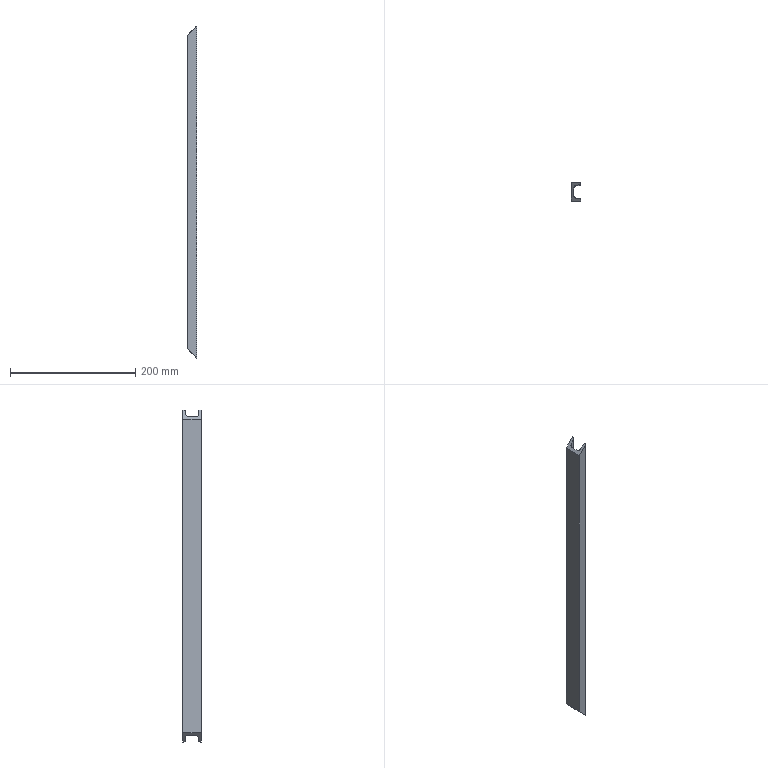Part | STEP file | DIN 1026-1 U 30x15 1785506883170 | 1 solid | 14 faces | box 15 x 30 x 530 mm | volume 112916 mm3 | plane 10 | cylinder 4 | commonest cylinder face diameters 4 x2 9 x2
STEP:
#1=CARTESIAN_POINT('',(13.159,10.953,-13.159));
#2=VERTEX_POINT('',#1);
#3=CARTESIAN_POINT('',(15.,12.946,-15.));
#4=VERTEX_POINT('',#3);
#5=CARTESIAN_POINT('',(13.,12.946,-13.));
#6=DIRECTION('',(0.7071,0.,0.7071));
#7=DIRECTION('',(-0.7071,0.,0.7071));
#8=AXIS2_PLACEMENT_3D('',#5,#6,#7);
#9=ELLIPSE('',#8,2.828,2.);
#10=EDGE_CURVE('',#2,#4,#9,.T.);
#11=ORIENTED_EDGE('',*,*,#10,.F.);
#12=CARTESIAN_POINT('',(8.141,10.551,-8.141));
#13=VERTEX_POINT('',#12);
#14=CARTESIAN_POINT('',(3.103,10.148,-3.103));
#15=DIRECTION('',(0.706,0.05648,-0.706));
#16=VECTOR('',#15,10.);
#17=LINE('',#14,#16);
#18=EDGE_CURVE('',#13,#2,#17,.T.);
#19=ORIENTED_EDGE('',*,*,#18,.F.);
#20=CARTESIAN_POINT('',(4.,6.066,-4.));
#21=VERTEX_POINT('',#20);
#22=CARTESIAN_POINT('',(8.5,6.066,-8.5));
#23=DIRECTION('',(-0.7071,0.,-0.7071));
#24=DIRECTION('',(-0.7071,0.,0.7071));
#25=AXIS2_PLACEMENT_3D('',#22,#23,#24);
#26=ELLIPSE('',#25,6.364,4.5);
#27=EDGE_CURVE('',#21,#13,#26,.T.);
#28=ORIENTED_EDGE('',*,*,#27,.F.);
#29=CARTESIAN_POINT('',(4.,-6.066,-4.));
#30=VERTEX_POINT('',#29);
#31=CARTESIAN_POINT('',(4.,0.,-4.));
#32=DIRECTION('',(0.,1.,0.));
#33=VECTOR('',#32,10.);
#34=LINE('',#31,#33);
#35=EDGE_CURVE('',#30,#21,#34,.T.);
#36=ORIENTED_EDGE('',*,*,#35,.F.);
#37=CARTESIAN_POINT('',(8.141,-10.551,-8.141));
#38=VERTEX_POINT('',#37);
#39=CARTESIAN_POINT('',(8.5,-6.066,-8.5));
#40=DIRECTION('',(-0.7071,0.,-0.7071));
#41=DIRECTION('',(-0.7071,0.,0.7071));
#42=AXIS2_PLACEMENT_3D('',#39,#40,#41);
#43=ELLIPSE('',#42,6.364,4.5);
#44=EDGE_CURVE('',#38,#30,#43,.T.);
#45=ORIENTED_EDGE('',*,*,#44,.F.);
#46=CARTESIAN_POINT('',(13.159,-10.953,-13.159));
#47=VERTEX_POINT('',#46);
#48=CARTESIAN_POINT('',(1.844,-10.048,-1.844));
#49=DIRECTION('',(-0.706,0.05648,0.706));
#50=VECTOR('',#49,10.);
#51=LINE('',#48,#50);
#52=EDGE_CURVE('',#47,#38,#51,.T.);
#53=ORIENTED_EDGE('',*,*,#52,.F.);
#54=CARTESIAN_POINT('',(15.,-12.946,-15.));
#55=VERTEX_POINT('',#54);
#56=CARTESIAN_POINT('',(13.,-12.946,-13.));
#57=DIRECTION('',(0.7071,0.,0.7071));
#58=DIRECTION('',(-0.7071,0.,0.7071));
#59=AXIS2_PLACEMENT_3D('',#56,#57,#58);
#60=ELLIPSE('',#59,2.828,2.);
#61=EDGE_CURVE('',#55,#47,#60,.T.);
#62=ORIENTED_EDGE('',*,*,#61,.F.);
#63=CARTESIAN_POINT('',(15.,-15.,-15.));
#64=VERTEX_POINT('',#63);
#65=CARTESIAN_POINT('',(15.,-6.473,-15.));
#66=DIRECTION('',(0.,-1.,0.));
#67=VECTOR('',#66,10.);
#68=LINE('',#65,#67);
#69=EDGE_CURVE('',#55,#64,#68,.T.);
#70=ORIENTED_EDGE('',*,*,#69,.T.);
#71=CARTESIAN_POINT('',(0.,-15.,0.));
#72=VERTEX_POINT('',#71);
#73=CARTESIAN_POINT('',(3.75,-15.,-3.75));
#74=DIRECTION('',(0.7071,0.,-0.7071));
#75=VECTOR('',#74,10.);
#76=LINE('',#73,#75);
#77=EDGE_CURVE('',#72,#64,#76,.T.);
#78=ORIENTED_EDGE('',*,*,#77,.F.);
#79=CARTESIAN_POINT('',(0.,15.,0.));
#80=VERTEX_POINT('',#79);
#81=CARTESIAN_POINT('',(0.,0.,0.));
#82=DIRECTION('',(0.,-1.,0.));
#83=VECTOR('',#82,10.);
#84=LINE('',#81,#83);
#85=EDGE_CURVE('',#80,#72,#84,.T.);
#86=ORIENTED_EDGE('',*,*,#85,.F.);
#87=CARTESIAN_POINT('',(15.,15.,-15.));
#88=VERTEX_POINT('',#87);
#89=CARTESIAN_POINT('',(0.,15.,0.));
#90=DIRECTION('',(-0.7071,0.,0.7071));
#91=VECTOR('',#90,10.);
#92=LINE('',#89,#91);
#93=EDGE_CURVE('',#88,#80,#92,.T.);
#94=ORIENTED_EDGE('',*,*,#93,.F.);
#95=CARTESIAN_POINT('',(15.,7.5,-15.));
#96=DIRECTION('',(0.,-1.,0.));
#97=VECTOR('',#96,10.);
#98=LINE('',#95,#97);
#99=EDGE_CURVE('',#88,#4,#98,.T.);
#100=ORIENTED_EDGE('',*,*,#99,.T.);
#101=EDGE_LOOP('',(#11,#19,#28,#36,#45,#53,#62,#70,#78,#86,#94,#100));
#102=FACE_OUTER_BOUND('',#101,.T.);
#103=CARTESIAN_POINT('',(0.,0.,0.));
#104=DIRECTION('',(0.7071,0.,0.7071));
#105=DIRECTION('',(0.7071,0.,-0.7071));
#106=AXIS2_PLACEMENT_3D('',#103,#104,#105);
#107=PLANE('',#106);
#108=ADVANCED_FACE('',(#102),#107,.F.);
#109=ORIENTED_EDGE('',*,*,#61,.T.);
#110=CARTESIAN_POINT('',(13.159,-10.953,513.159));
#111=VERTEX_POINT('',#110);
#112=CARTESIAN_POINT('',(13.159,-10.953,0.));
#113=DIRECTION('',(0.,0.,-1.));
#114=VECTOR('',#113,10.);
#115=LINE('',#112,#114);
#116=EDGE_CURVE('',#111,#47,#115,.T.);
#117=ORIENTED_EDGE('',*,*,#116,.F.);
#118=CARTESIAN_POINT('',(15.,-12.946,515.));
#119=VERTEX_POINT('',#118);
#120=CARTESIAN_POINT('',(13.,-12.946,513.));
#121=DIRECTION('',(0.7071,0.,-0.7071));
#122=DIRECTION('',(-0.7071,0.,-0.7071));
#123=AXIS2_PLACEMENT_3D('',#120,#121,#122);
#124=ELLIPSE('',#123,2.828,2.);
#125=EDGE_CURVE('',#111,#119,#124,.T.);
#126=ORIENTED_EDGE('',*,*,#125,.T.);
#127=CARTESIAN_POINT('',(15.,-12.946,0.));
#128=DIRECTION('',(0.,0.,-1.));
#129=VECTOR('',#128,10.);
#130=LINE('',#127,#129);
#131=EDGE_CURVE('',#119,#55,#130,.T.);
#132=ORIENTED_EDGE('',*,*,#131,.T.);
#133=EDGE_LOOP('',(#109,#117,#126,#132));
#134=FACE_OUTER_BOUND('',#133,.T.);
#135=CARTESIAN_POINT('',(13.,-12.946,0.));
#136=DIRECTION('',(0.,0.,1.));
#137=DIRECTION('',(-1.,0.,0.));
#138=AXIS2_PLACEMENT_3D('',#135,#136,#137);
#139=CYLINDRICAL_SURFACE('',#138,2.);
#140=ADVANCED_FACE('',(#134),#139,.T.);
#141=ORIENTED_EDGE('',*,*,#52,.T.);
#142=CARTESIAN_POINT('',(8.141,-10.551,508.141));
#143=VERTEX_POINT('',#142);
#144=CARTESIAN_POINT('',(8.141,-10.551,0.));
#145=DIRECTION('',(0.,0.,-1.));
#146=VECTOR('',#145,10.);
#147=LINE('',#144,#146);
#148=EDGE_CURVE('',#143,#38,#147,.T.);
#149=ORIENTED_EDGE('',*,*,#148,.F.);
#150=CARTESIAN_POINT('',(-247.358,9.889,252.642));
#151=DIRECTION('',(0.706,-0.05648,0.706));
#152=VECTOR('',#151,10.);
#153=LINE('',#150,#152);
#154=EDGE_CURVE('',#143,#111,#153,.T.);
#155=ORIENTED_EDGE('',*,*,#154,.T.);
#156=ORIENTED_EDGE('',*,*,#116,.T.);
#157=EDGE_LOOP('',(#141,#149,#155,#156));
#158=FACE_OUTER_BOUND('',#157,.T.);
#159=CARTESIAN_POINT('',(8.141,-10.551,0.));
#160=DIRECTION('',(0.07975,0.9968,0.));
#161=DIRECTION('',(0.,0.,1.));
#162=AXIS2_PLACEMENT_3D('',#159,#160,#161);
#163=PLANE('',#162);
#164=ADVANCED_FACE('',(#158),#163,.T.);
#165=ORIENTED_EDGE('',*,*,#44,.T.);
#166=CARTESIAN_POINT('',(4.,-6.066,504.));
#167=VERTEX_POINT('',#166);
#168=CARTESIAN_POINT('',(4.,-6.066,0.));
#169=DIRECTION('',(0.,0.,-1.));
#170=VECTOR('',#169,10.);
#171=LINE('',#168,#170);
#172=EDGE_CURVE('',#167,#30,#171,.T.);
#173=ORIENTED_EDGE('',*,*,#172,.F.);
#174=CARTESIAN_POINT('',(8.5,-6.066,508.5));
#175=DIRECTION('',(-0.7071,0.,0.7071));
#176=DIRECTION('',(-0.7071,0.,-0.7071));
#177=AXIS2_PLACEMENT_3D('',#174,#175,#176);
#178=ELLIPSE('',#177,6.364,4.5);
#179=EDGE_CURVE('',#167,#143,#178,.T.);
#180=ORIENTED_EDGE('',*,*,#179,.T.);
#181=ORIENTED_EDGE('',*,*,#148,.T.);
#182=EDGE_LOOP('',(#165,#173,#180,#181));
#183=FACE_OUTER_BOUND('',#182,.T.);
#184=CARTESIAN_POINT('',(8.5,-6.066,0.));
#185=DIRECTION('',(0.,0.,1.));
#186=DIRECTION('',(-1.,0.,0.));
#187=AXIS2_PLACEMENT_3D('',#184,#185,#186);
#188=CYLINDRICAL_SURFACE('',#187,4.5);
#189=ADVANCED_FACE('',(#183),#188,.F.);
#190=ORIENTED_EDGE('',*,*,#35,.T.);
#191=CARTESIAN_POINT('',(4.,6.066,504.));
#192=VERTEX_POINT('',#191);
#193=CARTESIAN_POINT('',(4.,6.066,0.));
#194=DIRECTION('',(0.,0.,-1.));
#195=VECTOR('',#194,10.);
#196=LINE('',#193,#195);
#197=EDGE_CURVE('',#192,#21,#196,.T.);
#198=ORIENTED_EDGE('',*,*,#197,.F.);
#199=CARTESIAN_POINT('',(4.,0.,504.));
#200=DIRECTION('',(0.,-1.,0.));
#201=VECTOR('',#200,10.);
#202=LINE('',#199,#201);
#203=EDGE_CURVE('',#192,#167,#202,.T.);
#204=ORIENTED_EDGE('',*,*,#203,.T.);
#205=ORIENTED_EDGE('',*,*,#172,.T.);
#206=EDGE_LOOP('',(#190,#198,#204,#205));
#207=FACE_OUTER_BOUND('',#206,.T.);
#208=CARTESIAN_POINT('',(4.,0.,0.));
#209=DIRECTION('',(1.,0.,0.));
#210=DIRECTION('',(0.,0.,-1.));
#211=AXIS2_PLACEMENT_3D('',#208,#209,#210);
#212=PLANE('',#211);
#213=ADVANCED_FACE('',(#207),#212,.T.);
#214=ORIENTED_EDGE('',*,*,#27,.T.);
#215=CARTESIAN_POINT('',(8.141,10.551,508.141));
#216=VERTEX_POINT('',#215);
#217=CARTESIAN_POINT('',(8.141,10.551,0.));
#218=DIRECTION('',(0.,0.,-1.));
#219=VECTOR('',#218,10.);
#220=LINE('',#217,#219);
#221=EDGE_CURVE('',#216,#13,#220,.T.);
#222=ORIENTED_EDGE('',*,*,#221,.F.);
#223=CARTESIAN_POINT('',(8.5,6.066,508.5));
#224=DIRECTION('',(-0.7071,0.,0.7071));
#225=DIRECTION('',(-0.7071,0.,-0.7071));
#226=AXIS2_PLACEMENT_3D('',#223,#224,#225);
#227=ELLIPSE('',#226,6.364,4.5);
#228=EDGE_CURVE('',#216,#192,#227,.T.);
#229=ORIENTED_EDGE('',*,*,#228,.T.);
#230=ORIENTED_EDGE('',*,*,#197,.T.);
#231=EDGE_LOOP('',(#214,#222,#229,#230));
#232=FACE_OUTER_BOUND('',#231,.T.);
#233=CARTESIAN_POINT('',(8.5,6.066,0.));
#234=DIRECTION('',(0.,0.,1.));
#235=DIRECTION('',(-0.07975,0.9968,0.));
#236=AXIS2_PLACEMENT_3D('',#233,#234,#235);
#237=CYLINDRICAL_SURFACE('',#236,4.5);
#238=ADVANCED_FACE('',(#232),#237,.F.);
#239=ORIENTED_EDGE('',*,*,#18,.T.);
#240=CARTESIAN_POINT('',(13.159,10.953,513.159));
#241=VERTEX_POINT('',#240);
#242=CARTESIAN_POINT('',(13.159,10.953,0.));
#243=DIRECTION('',(0.,0.,-1.));
#244=VECTOR('',#243,10.);
#245=LINE('',#242,#244);
#246=EDGE_CURVE('',#241,#2,#245,.T.);
#247=ORIENTED_EDGE('',*,*,#246,.F.);
#248=CARTESIAN_POINT('',(-246.1,-9.788,253.9));
#249=DIRECTION('',(-0.706,-0.05648,-0.706));
#250=VECTOR('',#249,10.);
#251=LINE('',#248,#250);
#252=EDGE_CURVE('',#241,#216,#251,.T.);
#253=ORIENTED_EDGE('',*,*,#252,.T.);
#254=ORIENTED_EDGE('',*,*,#221,.T.);
#255=EDGE_LOOP('',(#239,#247,#253,#254));
#256=FACE_OUTER_BOUND('',#255,.T.);
#257=CARTESIAN_POINT('',(13.159,10.953,0.));
#258=DIRECTION('',(0.07975,-0.9968,0.));
#259=DIRECTION('',(0.,0.,-1.));
#260=AXIS2_PLACEMENT_3D('',#257,#258,#259);
#261=PLANE('',#260);
#262=ADVANCED_FACE('',(#256),#261,.T.);
#263=ORIENTED_EDGE('',*,*,#179,.F.);
#264=ORIENTED_EDGE('',*,*,#203,.F.);
#265=ORIENTED_EDGE('',*,*,#228,.F.);
#266=ORIENTED_EDGE('',*,*,#252,.F.);
#267=CARTESIAN_POINT('',(15.,12.946,515.));
#268=VERTEX_POINT('',#267);
#269=CARTESIAN_POINT('',(13.,12.946,513.));
#270=DIRECTION('',(0.7071,0.,-0.7071));
#271=DIRECTION('',(-0.7071,0.,-0.7071));
#272=AXIS2_PLACEMENT_3D('',#269,#270,#271);
#273=ELLIPSE('',#272,2.828,2.);
#274=EDGE_CURVE('',#268,#241,#273,.T.);
#275=ORIENTED_EDGE('',*,*,#274,.F.);
#276=CARTESIAN_POINT('',(15.,15.,515.));
#277=VERTEX_POINT('',#276);
#278=CARTESIAN_POINT('',(15.,7.5,515.));
#279=DIRECTION('',(0.,-1.,0.));
#280=VECTOR('',#279,10.);
#281=LINE('',#278,#280);
#282=EDGE_CURVE('',#277,#268,#281,.T.);
#283=ORIENTED_EDGE('',*,*,#282,.F.);
#284=CARTESIAN_POINT('',(0.,15.,500.));
#285=VERTEX_POINT('',#284);
#286=CARTESIAN_POINT('',(-250.,15.,250.));
#287=DIRECTION('',(0.7071,0.,0.7071));
#288=VECTOR('',#287,10.);
#289=LINE('',#286,#288);
#290=EDGE_CURVE('',#285,#277,#289,.T.);
#291=ORIENTED_EDGE('',*,*,#290,.F.);
#292=CARTESIAN_POINT('',(0.,-15.,500.));
#293=VERTEX_POINT('',#292);
#294=CARTESIAN_POINT('',(0.,0.,500.));
#295=DIRECTION('',(0.,1.,0.));
#296=VECTOR('',#295,10.);
#297=LINE('',#294,#296);
#298=EDGE_CURVE('',#293,#285,#297,.T.);
#299=ORIENTED_EDGE('',*,*,#298,.F.);
#300=CARTESIAN_POINT('',(15.,-15.,515.));
#301=VERTEX_POINT('',#300);
#302=CARTESIAN_POINT('',(-246.25,-15.,253.75));
#303=DIRECTION('',(-0.7071,0.,-0.7071));
#304=VECTOR('',#303,10.);
#305=LINE('',#302,#304);
#306=EDGE_CURVE('',#301,#293,#305,.T.);
#307=ORIENTED_EDGE('',*,*,#306,.F.);
#308=CARTESIAN_POINT('',(15.,-6.473,515.));
#309=DIRECTION('',(0.,-1.,0.));
#310=VECTOR('',#309,10.);
#311=LINE('',#308,#310);
#312=EDGE_CURVE('',#119,#301,#311,.T.);
#313=ORIENTED_EDGE('',*,*,#312,.F.);
#314=ORIENTED_EDGE('',*,*,#125,.F.);
#315=ORIENTED_EDGE('',*,*,#154,.F.);
#316=EDGE_LOOP('',(#263,#264,#265,#266,#275,#283,#291,#299,#307,#313,#314,#315));
#317=FACE_OUTER_BOUND('',#316,.T.);
#318=CARTESIAN_POINT('',(-250.,0.,250.));
#319=DIRECTION('',(0.7071,0.,-0.7071));
#320=DIRECTION('',(-0.7071,0.,-0.7071));
#321=AXIS2_PLACEMENT_3D('',#318,#319,#320);
#322=PLANE('',#321);
#323=ADVANCED_FACE('',(#317),#322,.F.);
#324=ORIENTED_EDGE('',*,*,#93,.T.);
#325=CARTESIAN_POINT('',(0.,15.,0.));
#326=DIRECTION('',(0.,0.,-1.));
#327=VECTOR('',#326,10.);
#328=LINE('',#325,#327);
#329=EDGE_CURVE('',#285,#80,#328,.T.);
#330=ORIENTED_EDGE('',*,*,#329,.F.);
#331=ORIENTED_EDGE('',*,*,#290,.T.);
#332=CARTESIAN_POINT('',(15.,15.,0.));
#333=DIRECTION('',(0.,0.,-1.));
#334=VECTOR('',#333,10.);
#335=LINE('',#332,#334);
#336=EDGE_CURVE('',#277,#88,#335,.T.);
#337=ORIENTED_EDGE('',*,*,#336,.T.);
#338=EDGE_LOOP('',(#324,#330,#331,#337));
#339=FACE_OUTER_BOUND('',#338,.T.);
#340=CARTESIAN_POINT('',(0.,15.,0.));
#341=DIRECTION('',(0.,1.,0.));
#342=DIRECTION('',(0.,0.,1.));
#343=AXIS2_PLACEMENT_3D('',#340,#341,#342);
#344=PLANE('',#343);
#345=ADVANCED_FACE('',(#339),#344,.T.);
#346=ORIENTED_EDGE('',*,*,#10,.T.);
#347=CARTESIAN_POINT('',(15.,12.946,0.));
#348=DIRECTION('',(0.,0.,-1.));
#349=VECTOR('',#348,10.);
#350=LINE('',#347,#349);
#351=EDGE_CURVE('',#268,#4,#350,.T.);
#352=ORIENTED_EDGE('',*,*,#351,.F.);
#353=ORIENTED_EDGE('',*,*,#274,.T.);
#354=ORIENTED_EDGE('',*,*,#246,.T.);
#355=EDGE_LOOP('',(#346,#352,#353,#354));
#356=FACE_OUTER_BOUND('',#355,.T.);
#357=CARTESIAN_POINT('',(13.,12.946,0.));
#358=DIRECTION('',(0.,0.,1.));
#359=DIRECTION('',(-0.07975,0.9968,0.));
#360=AXIS2_PLACEMENT_3D('',#357,#358,#359);
#361=CYLINDRICAL_SURFACE('',#360,2.);
#362=ADVANCED_FACE('',(#356),#361,.T.);
#363=ORIENTED_EDGE('',*,*,#312,.T.);
#364=CARTESIAN_POINT('',(15.,-15.,0.));
#365=DIRECTION('',(0.,0.,-1.));
#366=VECTOR('',#365,10.);
#367=LINE('',#364,#366);
#368=EDGE_CURVE('',#301,#64,#367,.T.);
#369=ORIENTED_EDGE('',*,*,#368,.T.);
#370=ORIENTED_EDGE('',*,*,#69,.F.);
#371=ORIENTED_EDGE('',*,*,#131,.F.);
#372=EDGE_LOOP('',(#363,#369,#370,#371));
#373=FACE_OUTER_BOUND('',#372,.T.);
#374=CARTESIAN_POINT('',(15.,-12.946,0.));
#375=DIRECTION('',(1.,0.,0.));
#376=DIRECTION('',(0.,0.,-1.));
#377=AXIS2_PLACEMENT_3D('',#374,#375,#376);
#378=PLANE('',#377);
#379=ADVANCED_FACE('',(#373),#378,.T.);
#380=ORIENTED_EDGE('',*,*,#77,.T.);
#381=ORIENTED_EDGE('',*,*,#368,.F.);
#382=ORIENTED_EDGE('',*,*,#306,.T.);
#383=CARTESIAN_POINT('',(0.,-15.,0.));
#384=DIRECTION('',(0.,0.,-1.));
#385=VECTOR('',#384,10.);
#386=LINE('',#383,#385);
#387=EDGE_CURVE('',#293,#72,#386,.T.);
#388=ORIENTED_EDGE('',*,*,#387,.T.);
#389=EDGE_LOOP('',(#380,#381,#382,#388));
#390=FACE_OUTER_BOUND('',#389,.T.);
#391=CARTESIAN_POINT('',(15.,-15.,0.));
#392=DIRECTION('',(0.,-1.,0.));
#393=DIRECTION('',(0.,0.,-1.));
#394=AXIS2_PLACEMENT_3D('',#391,#392,#393);
#395=PLANE('',#394);
#396=ADVANCED_FACE('',(#390),#395,.T.);
#397=ORIENTED_EDGE('',*,*,#85,.T.);
#398=ORIENTED_EDGE('',*,*,#387,.F.);
#399=ORIENTED_EDGE('',*,*,#298,.T.);
#400=ORIENTED_EDGE('',*,*,#329,.T.);
#401=EDGE_LOOP('',(#397,#398,#399,#400));
#402=FACE_OUTER_BOUND('',#401,.T.);
#403=CARTESIAN_POINT('',(0.,0.,0.));
#404=DIRECTION('',(-1.,0.,0.));
#405=DIRECTION('',(0.,0.,1.));
#406=AXIS2_PLACEMENT_3D('',#403,#404,#405);
#407=PLANE('',#406);
#408=ADVANCED_FACE('',(#402),#407,.T.);
#409=ORIENTED_EDGE('',*,*,#282,.T.);
#410=ORIENTED_EDGE('',*,*,#351,.T.);
#411=ORIENTED_EDGE('',*,*,#99,.F.);
#412=ORIENTED_EDGE('',*,*,#336,.F.);
#413=EDGE_LOOP('',(#409,#410,#411,#412));
#414=FACE_OUTER_BOUND('',#413,.T.);
#415=CARTESIAN_POINT('',(15.,15.,0.));
#416=DIRECTION('',(1.,0.,0.));
#417=DIRECTION('',(0.,0.,-1.));
#418=AXIS2_PLACEMENT_3D('',#415,#416,#417);
#419=PLANE('',#418);
#420=ADVANCED_FACE('',(#414),#419,.T.);
#421=CLOSED_SHELL('',(#108,#140,#164,#189,#213,#238,#262,#323,#345,#362,#379,#396,#408,#420));
#422=MANIFOLD_SOLID_BREP('',#421);
#423=(LENGTH_UNIT()NAMED_UNIT(*)SI_UNIT(.MILLI.,.METRE.));
#424=UNCERTAINTY_MEASURE_WITH_UNIT(LENGTH_MEASURE(0.01),#423,'','');
#425=(NAMED_UNIT(*)PLANE_ANGLE_UNIT()SI_UNIT($,.RADIAN.));
#426=(NAMED_UNIT(*)SI_UNIT($,.STERADIAN.)SOLID_ANGLE_UNIT());
#427=(GEOMETRIC_REPRESENTATION_CONTEXT(3)GLOBAL_UNCERTAINTY_ASSIGNED_CONTEXT((#424))GLOBAL_UNIT_ASSIGNED_CONTEXT((#423,#425,#426))REPRESENTATION_CONTEXT('',''));
#428=ADVANCED_BREP_SHAPE_REPRESENTATION('',(#422),#427);